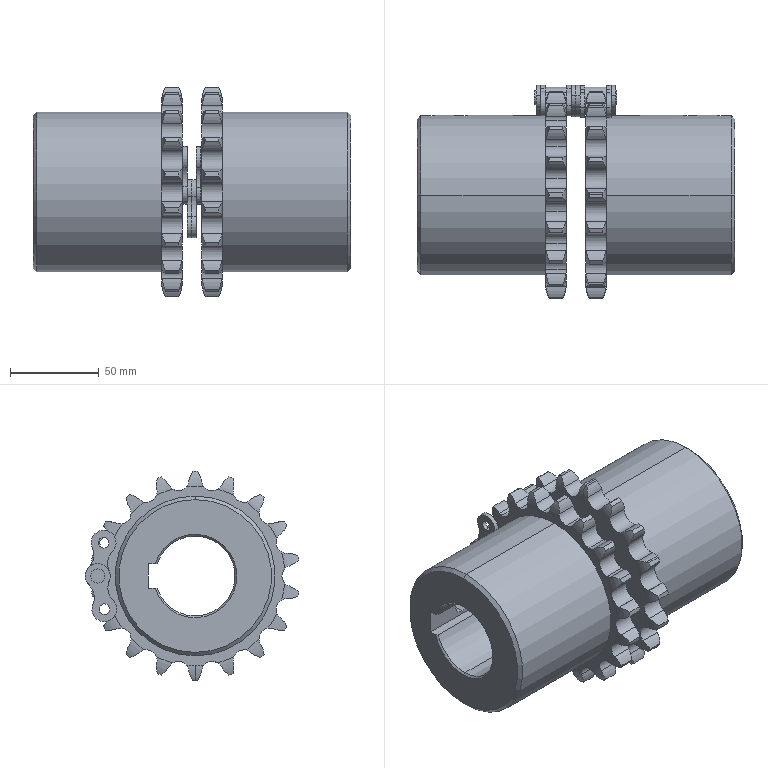Part | SolidWorks | features CompositeCurve 3 | 13 solids | 392 faces | box 178.9 x 120.134 x 117.94 mm | volume 822533 mm3 | cylinder 266 | torus 76 | plane 34 | cone 16 | commonest cylinder face diameters 28 x80 11.91 x56 6 x36 14 x24 117.9 x19 117.94 x19